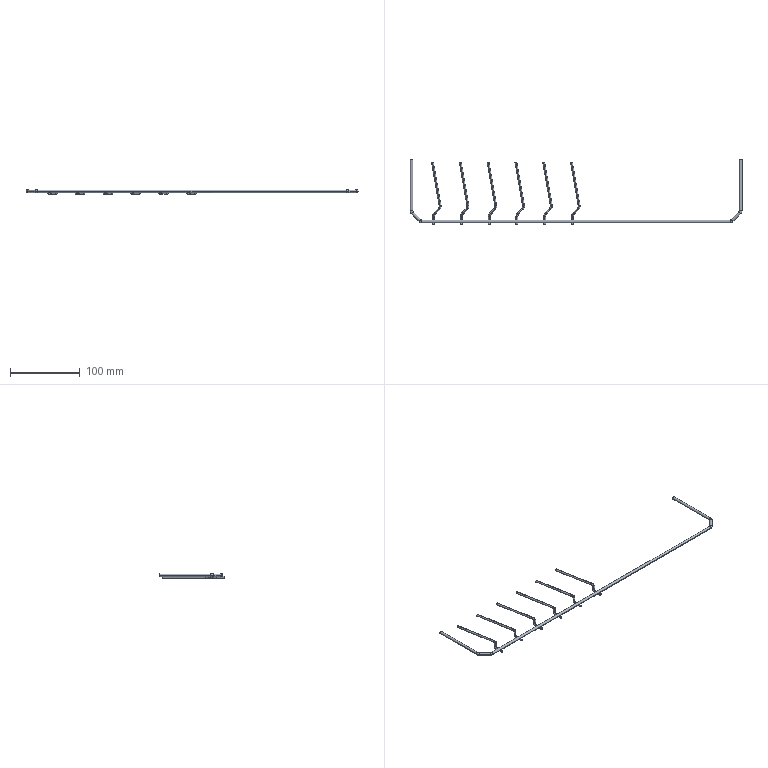Part | STEP file | ZXW722-L-178_XIAGEJIA_19_1_2_2_ | 1 solid | 92 faces | box 477.6 x 93 x 6.2 mm | volume 11029 mm3 | cylinder 46 | torus 32 | plane 14 | commonest cylinder face diameters 2.8 x36 3.9 x10